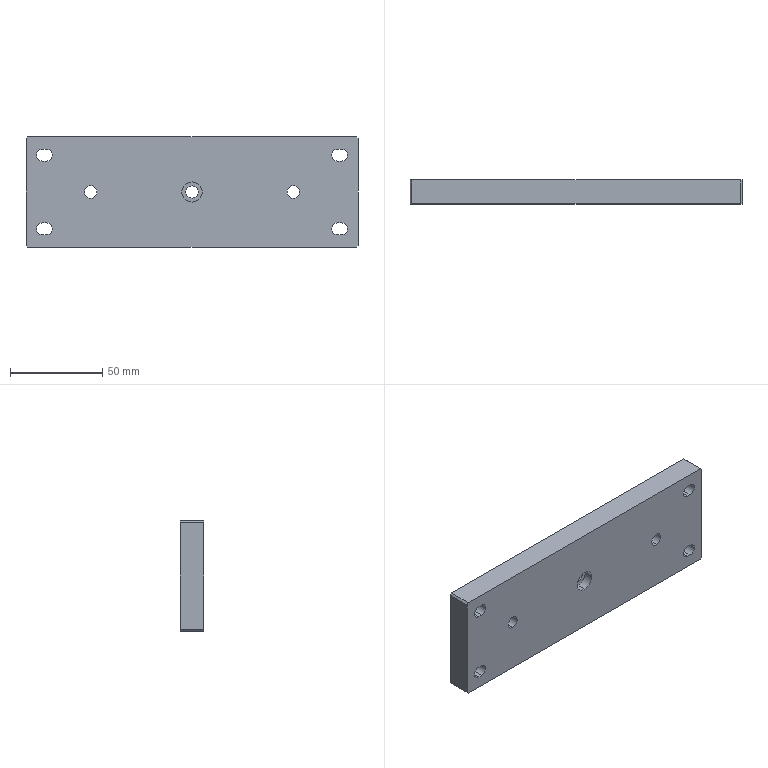Part | STEP file | PN_0014 Plate 2_Default | 1 solid | 38 faces | box 180 x 13 x 60 mm | volume 135779 mm3 | plane 20 | cylinder 18 | commonest cylinder face diameters 6.5 x8 6.8 x4 6.6 x2 11 x2 16 x2